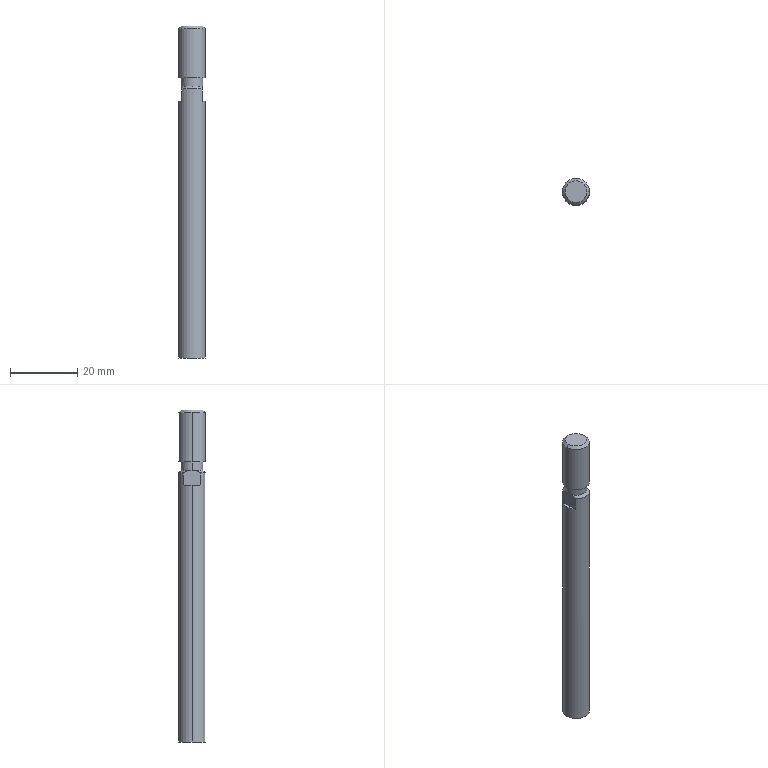Part | NX | features BREP 1 | 1 solid | 19 faces | box 8 x 8 x 99 mm | volume 4889 mm3 | plane 9 | cylinder 6 | cone 4 | commonest cylinder face diameters 8 x4 6.47 x2
STEP:
#1=CARTESIAN_POINT('',(3.,2.646,0.5));
#2=VERTEX_POINT('',#1);
#3=CARTESIAN_POINT('',(4.,0.,0.5));
#4=VERTEX_POINT('',#3);
#5=CARTESIAN_POINT('',(0.,0.,0.5));
#6=DIRECTION('',(0.,0.,-1.));
#7=DIRECTION('',(-1.,0.,0.));
#8=AXIS2_PLACEMENT_3D('',#5,#6,#7);
#9=CIRCLE('',#8,4.);
#10=EDGE_CURVE('',#2,#4,#9,.T.);
#11=ORIENTED_EDGE('',*,*,#10,.T.);
#12=CARTESIAN_POINT('',(4.,0.,-76.));
#13=VERTEX_POINT('',#12);
#14=CARTESIAN_POINT('',(4.,0.,-35.883));
#15=DIRECTION('',(0.,0.,-1.));
#16=VECTOR('',#15,1000.);
#17=LINE('',#14,#16);
#18=EDGE_CURVE('',#4,#13,#17,.T.);
#19=ORIENTED_EDGE('',*,*,#18,.T.);
#20=CARTESIAN_POINT('',(-4.,0.,-76.));
#21=VERTEX_POINT('',#20);
#22=CARTESIAN_POINT('',(0.,0.,-76.));
#23=DIRECTION('',(0.,0.,1.));
#24=DIRECTION('',(-1.,0.,0.));
#25=AXIS2_PLACEMENT_3D('',#22,#23,#24);
#26=CIRCLE('',#25,4.);
#27=EDGE_CURVE('',#13,#21,#26,.T.);
#28=ORIENTED_EDGE('',*,*,#27,.T.);
#29=CARTESIAN_POINT('',(-4.,0.,0.5));
#30=VERTEX_POINT('',#29);
#31=CARTESIAN_POINT('',(-4.,0.,-35.883));
#32=DIRECTION('',(0.,0.,-1.));
#33=VECTOR('',#32,1000.);
#34=LINE('',#31,#33);
#35=EDGE_CURVE('',#30,#21,#34,.T.);
#36=ORIENTED_EDGE('',*,*,#35,.F.);
#37=CARTESIAN_POINT('',(-3.,2.646,0.5));
#38=VERTEX_POINT('',#37);
#39=CARTESIAN_POINT('',(0.,0.,0.5));
#40=DIRECTION('',(0.,0.,-1.));
#41=DIRECTION('',(-1.,0.,0.));
#42=AXIS2_PLACEMENT_3D('',#39,#40,#41);
#43=CIRCLE('',#42,4.);
#44=EDGE_CURVE('',#30,#38,#43,.T.);
#45=ORIENTED_EDGE('',*,*,#44,.T.);
#46=CARTESIAN_POINT('',(-3.,2.646,4.235));
#47=VERTEX_POINT('',#46);
#48=CARTESIAN_POINT('',(-3.,2.646,-35.883));
#49=DIRECTION('',(0.,0.,1.));
#50=VECTOR('',#49,1000.);
#51=LINE('',#48,#50);
#52=EDGE_CURVE('',#38,#47,#51,.T.);
#53=ORIENTED_EDGE('',*,*,#52,.T.);
#54=CARTESIAN_POINT('',(3.,2.646,4.235));
#55=VERTEX_POINT('',#54);
#56=CARTESIAN_POINT('',(0.,0.,4.235));
#57=DIRECTION('',(0.,0.,-1.));
#58=DIRECTION('',(-1.,0.,0.));
#59=AXIS2_PLACEMENT_3D('',#56,#57,#58);
#60=CIRCLE('',#59,4.);
#61=EDGE_CURVE('',#47,#55,#60,.T.);
#62=ORIENTED_EDGE('',*,*,#61,.T.);
#63=CARTESIAN_POINT('',(3.,2.646,-35.883));
#64=DIRECTION('',(0.,0.,-1.));
#65=VECTOR('',#64,1000.);
#66=LINE('',#63,#65);
#67=EDGE_CURVE('',#55,#2,#66,.T.);
#68=ORIENTED_EDGE('',*,*,#67,.T.);
#69=EDGE_LOOP('',(#11,#19,#28,#36,#45,#53,#62,#68));
#70=FACE_BOUND('',#69,.T.);
#71=CARTESIAN_POINT('',(0.,0.,-35.883));
#72=DIRECTION('',(0.,0.,-1.));
#73=DIRECTION('',(-1.,0.,0.));
#74=AXIS2_PLACEMENT_3D('',#71,#72,#73);
#75=CYLINDRICAL_SURFACE('',#74,4.);
#76=ADVANCED_FACE('',(#70),#75,.T.);
#77=CARTESIAN_POINT('',(-3.235,0.,7.5));
#78=VERTEX_POINT('',#77);
#79=CARTESIAN_POINT('',(3.235,0.,7.5));
#80=VERTEX_POINT('',#79);
#81=CARTESIAN_POINT('',(0.,0.,7.5));
#82=DIRECTION('',(0.,0.,-1.));
#83=DIRECTION('',(-1.,0.,0.));
#84=AXIS2_PLACEMENT_3D('',#81,#82,#83);
#85=CIRCLE('',#84,3.235);
#86=EDGE_CURVE('',#78,#80,#85,.T.);
#87=ORIENTED_EDGE('',*,*,#86,.T.);
#88=CARTESIAN_POINT('',(3.235,0.,5.));
#89=VERTEX_POINT('',#88);
#90=CARTESIAN_POINT('',(3.235,0.,6.25));
#91=DIRECTION('',(0.,0.,-1.));
#92=VECTOR('',#91,1000.);
#93=LINE('',#90,#92);
#94=EDGE_CURVE('',#80,#89,#93,.T.);
#95=ORIENTED_EDGE('',*,*,#94,.T.);
#96=CARTESIAN_POINT('',(3.,1.21,5.));
#97=VERTEX_POINT('',#96);
#98=CARTESIAN_POINT('',(0.,0.,5.));
#99=DIRECTION('',(0.,0.,1.));
#100=DIRECTION('',(-1.,0.,0.));
#101=AXIS2_PLACEMENT_3D('',#98,#99,#100);
#102=CIRCLE('',#101,3.235);
#103=EDGE_CURVE('',#89,#97,#102,.T.);
#104=ORIENTED_EDGE('',*,*,#103,.T.);
#105=CARTESIAN_POINT('',(-3.,1.21,5.));
#106=VERTEX_POINT('',#105);
#107=CARTESIAN_POINT('',(0.,0.,5.));
#108=DIRECTION('',(0.,0.,-1.));
#109=DIRECTION('',(0.,1.,0.));
#110=AXIS2_PLACEMENT_3D('',#107,#108,#109);
#111=CIRCLE('',#110,3.235);
#112=EDGE_CURVE('',#106,#97,#111,.T.);
#113=ORIENTED_EDGE('',*,*,#112,.F.);
#114=CARTESIAN_POINT('',(-3.235,0.,5.));
#115=VERTEX_POINT('',#114);
#116=CARTESIAN_POINT('',(0.,0.,5.));
#117=DIRECTION('',(0.,0.,1.));
#118=DIRECTION('',(-1.,0.,0.));
#119=AXIS2_PLACEMENT_3D('',#116,#117,#118);
#120=CIRCLE('',#119,3.235);
#121=EDGE_CURVE('',#106,#115,#120,.T.);
#122=ORIENTED_EDGE('',*,*,#121,.T.);
#123=CARTESIAN_POINT('',(-3.235,0.,6.25));
#124=DIRECTION('',(0.,0.,-1.));
#125=VECTOR('',#124,1000.);
#126=LINE('',#123,#125);
#127=EDGE_CURVE('',#78,#115,#126,.T.);
#128=ORIENTED_EDGE('',*,*,#127,.F.);
#129=EDGE_LOOP('',(#87,#95,#104,#113,#122,#128));
#130=FACE_BOUND('',#129,.T.);
#131=CARTESIAN_POINT('',(0.,0.,6.25));
#132=DIRECTION('',(0.,0.,-1.));
#133=DIRECTION('',(-1.,0.,0.));
#134=AXIS2_PLACEMENT_3D('',#131,#132,#133);
#135=CYLINDRICAL_SURFACE('',#134,3.235);
#136=ADVANCED_FACE('',(#130),#135,.T.);
#137=CARTESIAN_POINT('',(-4.,0.,22.235));
#138=VERTEX_POINT('',#137);
#139=CARTESIAN_POINT('',(4.,0.,22.235));
#140=VERTEX_POINT('',#139);
#141=CARTESIAN_POINT('',(0.,0.,22.235));
#142=DIRECTION('',(0.,0.,-1.));
#143=DIRECTION('',(-1.,0.,0.));
#144=AXIS2_PLACEMENT_3D('',#141,#142,#143);
#145=CIRCLE('',#144,4.);
#146=EDGE_CURVE('',#138,#140,#145,.T.);
#147=ORIENTED_EDGE('',*,*,#146,.T.);
#148=CARTESIAN_POINT('',(4.,0.,7.5));
#149=VERTEX_POINT('',#148);
#150=CARTESIAN_POINT('',(4.,0.,14.867));
#151=DIRECTION('',(0.,0.,-1.));
#152=VECTOR('',#151,1000.);
#153=LINE('',#150,#152);
#154=EDGE_CURVE('',#140,#149,#153,.T.);
#155=ORIENTED_EDGE('',*,*,#154,.T.);
#156=CARTESIAN_POINT('',(-4.,0.,7.5));
#157=VERTEX_POINT('',#156);
#158=CARTESIAN_POINT('',(0.,0.,7.5));
#159=DIRECTION('',(0.,0.,-1.));
#160=DIRECTION('',(-1.,0.,0.));
#161=AXIS2_PLACEMENT_3D('',#158,#159,#160);
#162=CIRCLE('',#161,4.);
#163=EDGE_CURVE('',#157,#149,#162,.T.);
#164=ORIENTED_EDGE('',*,*,#163,.F.);
#165=CARTESIAN_POINT('',(-4.,0.,14.867));
#166=DIRECTION('',(0.,0.,-1.));
#167=VECTOR('',#166,1000.);
#168=LINE('',#165,#167);
#169=EDGE_CURVE('',#138,#157,#168,.T.);
#170=ORIENTED_EDGE('',*,*,#169,.F.);
#171=EDGE_LOOP('',(#147,#155,#164,#170));
#172=FACE_BOUND('',#171,.T.);
#173=CARTESIAN_POINT('',(0.,0.,14.867));
#174=DIRECTION('',(0.,0.,-1.));
#175=DIRECTION('',(-1.,0.,0.));
#176=AXIS2_PLACEMENT_3D('',#173,#174,#175);
#177=CYLINDRICAL_SURFACE('',#176,4.);
#178=ADVANCED_FACE('',(#172),#177,.T.);
#179=CARTESIAN_POINT('',(-3.235,0.,23.));
#180=VERTEX_POINT('',#179);
#181=CARTESIAN_POINT('',(3.235,0.,23.));
#182=VERTEX_POINT('',#181);
#183=CARTESIAN_POINT('',(0.,0.,23.));
#184=DIRECTION('',(0.,0.,-1.));
#185=DIRECTION('',(-1.,0.,0.));
#186=AXIS2_PLACEMENT_3D('',#183,#184,#185);
#187=CIRCLE('',#186,3.235);
#188=EDGE_CURVE('',#180,#182,#187,.T.);
#189=ORIENTED_EDGE('',*,*,#188,.T.);
#190=CARTESIAN_POINT('',(4.,0.,22.235));
#191=DIRECTION('',(0.7071,0.,-0.7071));
#192=VECTOR('',#191,1000.);
#193=LINE('',#190,#192);
#194=EDGE_CURVE('',#182,#140,#193,.T.);
#195=ORIENTED_EDGE('',*,*,#194,.T.);
#196=ORIENTED_EDGE('',*,*,#146,.F.);
#197=CARTESIAN_POINT('',(-4.,0.,22.235));
#198=DIRECTION('',(-0.7071,0.,-0.7071));
#199=VECTOR('',#198,1000.);
#200=LINE('',#197,#199);
#201=EDGE_CURVE('',#180,#138,#200,.T.);
#202=ORIENTED_EDGE('',*,*,#201,.F.);
#203=EDGE_LOOP('',(#189,#195,#196,#202));
#204=FACE_BOUND('',#203,.T.);
#205=CARTESIAN_POINT('',(0.,0.,22.235));
#206=DIRECTION('',(0.,0.,-1.));
#207=DIRECTION('',(-1.,0.,0.));
#208=AXIS2_PLACEMENT_3D('',#205,#206,#207);
#209=CONICAL_SURFACE('',#208,4.,0.7854);
#210=ADVANCED_FACE('',(#204),#209,.T.);
#211=ORIENTED_EDGE('',*,*,#18,.F.);
#212=CARTESIAN_POINT('',(3.,-2.646,0.5));
#213=VERTEX_POINT('',#212);
#214=CARTESIAN_POINT('',(0.,0.,0.5));
#215=DIRECTION('',(0.,0.,-1.));
#216=DIRECTION('',(-1.,0.,0.));
#217=AXIS2_PLACEMENT_3D('',#214,#215,#216);
#218=CIRCLE('',#217,4.);
#219=EDGE_CURVE('',#4,#213,#218,.T.);
#220=ORIENTED_EDGE('',*,*,#219,.T.);
#221=CARTESIAN_POINT('',(3.,-2.646,4.235));
#222=VERTEX_POINT('',#221);
#223=CARTESIAN_POINT('',(3.,-2.646,-35.883));
#224=DIRECTION('',(0.,0.,1.));
#225=VECTOR('',#224,1000.);
#226=LINE('',#223,#225);
#227=EDGE_CURVE('',#213,#222,#226,.T.);
#228=ORIENTED_EDGE('',*,*,#227,.T.);
#229=CARTESIAN_POINT('',(-3.,-2.646,4.235));
#230=VERTEX_POINT('',#229);
#231=CARTESIAN_POINT('',(0.,0.,4.235));
#232=DIRECTION('',(0.,0.,-1.));
#233=DIRECTION('',(-1.,0.,0.));
#234=AXIS2_PLACEMENT_3D('',#231,#232,#233);
#235=CIRCLE('',#234,4.);
#236=EDGE_CURVE('',#222,#230,#235,.T.);
#237=ORIENTED_EDGE('',*,*,#236,.T.);
#238=CARTESIAN_POINT('',(-3.,-2.646,0.5));
#239=VERTEX_POINT('',#238);
#240=CARTESIAN_POINT('',(-3.,-2.646,-35.883));
#241=DIRECTION('',(0.,0.,-1.));
#242=VECTOR('',#241,1000.);
#243=LINE('',#240,#242);
#244=EDGE_CURVE('',#230,#239,#243,.T.);
#245=ORIENTED_EDGE('',*,*,#244,.T.);
#246=CARTESIAN_POINT('',(0.,0.,0.5));
#247=DIRECTION('',(0.,0.,-1.));
#248=DIRECTION('',(-1.,0.,0.));
#249=AXIS2_PLACEMENT_3D('',#246,#247,#248);
#250=CIRCLE('',#249,4.);
#251=EDGE_CURVE('',#239,#30,#250,.T.);
#252=ORIENTED_EDGE('',*,*,#251,.T.);
#253=ORIENTED_EDGE('',*,*,#35,.T.);
#254=CARTESIAN_POINT('',(0.,0.,-76.));
#255=DIRECTION('',(0.,0.,1.));
#256=DIRECTION('',(-1.,0.,0.));
#257=AXIS2_PLACEMENT_3D('',#254,#255,#256);
#258=CIRCLE('',#257,4.);
#259=EDGE_CURVE('',#21,#13,#258,.T.);
#260=ORIENTED_EDGE('',*,*,#259,.T.);
#261=EDGE_LOOP('',(#211,#220,#228,#237,#245,#252,#253,#260));
#262=FACE_BOUND('',#261,.T.);
#263=CARTESIAN_POINT('',(0.,0.,-35.883));
#264=DIRECTION('',(0.,0.,-1.));
#265=DIRECTION('',(-1.,0.,0.));
#266=AXIS2_PLACEMENT_3D('',#263,#264,#265);
#267=CYLINDRICAL_SURFACE('',#266,4.);
#268=ADVANCED_FACE('',(#262),#267,.T.);
#269=CARTESIAN_POINT('',(-3.,1.21,5.));
#270=CARTESIAN_POINT('',(-3.,1.653,4.834));
#271=CARTESIAN_POINT('',(-3.,2.119,4.584));
#272=CARTESIAN_POINT('',(-3.,2.646,4.235));
#273=B_SPLINE_CURVE_WITH_KNOTS('',3,(#269,#270,#271,#272),.UNSPECIFIED.,.F.,.F.,(4,4),(0.,1.),.UNSPECIFIED.);
#274=EDGE_CURVE('',#47,#106,#273,.F.);
#275=ORIENTED_EDGE('',*,*,#274,.T.);
#276=ORIENTED_EDGE('',*,*,#112,.T.);
#277=CARTESIAN_POINT('',(3.,2.646,4.235));
#278=CARTESIAN_POINT('',(3.,2.12,4.583));
#279=CARTESIAN_POINT('',(3.,1.654,4.834));
#280=CARTESIAN_POINT('',(3.,1.21,5.));
#281=B_SPLINE_CURVE_WITH_KNOTS('',3,(#277,#278,#279,#280),.UNSPECIFIED.,.F.,.F.,(4,4),(0.,1.),.UNSPECIFIED.);
#282=EDGE_CURVE('',#97,#55,#281,.F.);
#283=ORIENTED_EDGE('',*,*,#282,.T.);
#284=ORIENTED_EDGE('',*,*,#61,.F.);
#285=EDGE_LOOP('',(#275,#276,#283,#284));
#286=FACE_BOUND('',#285,.T.);
#287=CARTESIAN_POINT('',(0.,0.,4.235));
#288=DIRECTION('',(0.,0.,-1.));
#289=DIRECTION('',(-1.,0.,0.));
#290=AXIS2_PLACEMENT_3D('',#287,#288,#289);
#291=CONICAL_SURFACE('',#290,4.,0.7854);
#292=ADVANCED_FACE('',(#286),#291,.T.);
#293=CARTESIAN_POINT('',(-3.,-1.21,5.));
#294=VERTEX_POINT('',#293);
#295=CARTESIAN_POINT('',(-3.,8.,5.));
#296=DIRECTION('',(0.,-1.,0.));
#297=VECTOR('',#296,1000.);
#298=LINE('',#295,#297);
#299=EDGE_CURVE('',#106,#294,#298,.T.);
#300=ORIENTED_EDGE('',*,*,#299,.F.);
#301=ORIENTED_EDGE('',*,*,#274,.F.);
#302=ORIENTED_EDGE('',*,*,#52,.F.);
#303=CARTESIAN_POINT('',(-3.,8.,0.5));
#304=DIRECTION('',(0.,1.,0.));
#305=VECTOR('',#304,1000.);
#306=LINE('',#303,#305);
#307=EDGE_CURVE('',#239,#38,#306,.T.);
#308=ORIENTED_EDGE('',*,*,#307,.F.);
#309=ORIENTED_EDGE('',*,*,#244,.F.);
#310=CARTESIAN_POINT('',(-3.,-2.646,4.235));
#311=CARTESIAN_POINT('',(-3.,-2.12,4.583));
#312=CARTESIAN_POINT('',(-3.,-1.654,4.834));
#313=CARTESIAN_POINT('',(-3.,-1.21,5.));
#314=B_SPLINE_CURVE_WITH_KNOTS('',3,(#310,#311,#312,#313),.UNSPECIFIED.,.F.,.F.,(4,4),(0.,1.),.UNSPECIFIED.);
#315=EDGE_CURVE('',#294,#230,#314,.F.);
#316=ORIENTED_EDGE('',*,*,#315,.F.);
#317=EDGE_LOOP('',(#300,#301,#302,#308,#309,#316));
#318=FACE_BOUND('',#317,.T.);
#319=CARTESIAN_POINT('',(-3.,8.,5.));
#320=DIRECTION('',(1.,0.,0.));
#321=DIRECTION('',(0.,1.,0.));
#322=AXIS2_PLACEMENT_3D('',#319,#320,#321);
#323=PLANE('',#322);
#324=ADVANCED_FACE('',(#318),#323,.F.);
#325=ORIENTED_EDGE('',*,*,#307,.T.);
#326=ORIENTED_EDGE('',*,*,#44,.F.);
#327=ORIENTED_EDGE('',*,*,#251,.F.);
#328=EDGE_LOOP('',(#325,#326,#327));
#329=FACE_BOUND('',#328,.T.);
#330=CARTESIAN_POINT('',(-3.,8.,0.5));
#331=DIRECTION('',(0.,0.,-1.));
#332=DIRECTION('',(0.,-1.,0.));
#333=AXIS2_PLACEMENT_3D('',#330,#331,#332);
#334=PLANE('',#333);
#335=ADVANCED_FACE('',(#329),#334,.F.);
#336=ORIENTED_EDGE('',*,*,#315,.T.);
#337=ORIENTED_EDGE('',*,*,#236,.F.);
#338=CARTESIAN_POINT('',(3.,-1.21,5.));
#339=VERTEX_POINT('',#338);
#340=CARTESIAN_POINT('',(3.,-1.21,5.));
#341=CARTESIAN_POINT('',(3.,-1.653,4.834));
#342=CARTESIAN_POINT('',(3.,-2.119,4.584));
#343=CARTESIAN_POINT('',(3.,-2.646,4.235));
#344=B_SPLINE_CURVE_WITH_KNOTS('',3,(#340,#341,#342,#343),.UNSPECIFIED.,.F.,.F.,(4,4),(0.,1.),.UNSPECIFIED.);
#345=EDGE_CURVE('',#222,#339,#344,.F.);
#346=ORIENTED_EDGE('',*,*,#345,.T.);
#347=CARTESIAN_POINT('',(0.,0.,5.));
#348=DIRECTION('',(0.,0.,-1.));
#349=DIRECTION('',(0.,1.,0.));
#350=AXIS2_PLACEMENT_3D('',#347,#348,#349);
#351=CIRCLE('',#350,3.235);
#352=EDGE_CURVE('',#339,#294,#351,.T.);
#353=ORIENTED_EDGE('',*,*,#352,.T.);
#354=EDGE_LOOP('',(#336,#337,#346,#353));
#355=FACE_BOUND('',#354,.T.);
#356=CARTESIAN_POINT('',(0.,0.,4.235));
#357=DIRECTION('',(0.,0.,-1.));
#358=DIRECTION('',(-1.,0.,0.));
#359=AXIS2_PLACEMENT_3D('',#356,#357,#358);
#360=CONICAL_SURFACE('',#359,4.,0.7854);
#361=ADVANCED_FACE('',(#355),#360,.T.);
#362=ORIENTED_EDGE('',*,*,#259,.F.);
#363=ORIENTED_EDGE('',*,*,#27,.F.);
#364=EDGE_LOOP('',(#362,#363));
#365=FACE_BOUND('',#364,.T.);
#366=CARTESIAN_POINT('',(0.,2.,-76.));
#367=DIRECTION('',(0.,0.,-1.));
#368=DIRECTION('',(0.,-1.,0.));
#369=AXIS2_PLACEMENT_3D('',#366,#367,#368);
#370=PLANE('',#369);
#371=ADVANCED_FACE('',(#365),#370,.T.);
#372=ORIENTED_EDGE('',*,*,#94,.F.);
#373=CARTESIAN_POINT('',(0.,0.,7.5));
#374=DIRECTION('',(0.,0.,-1.));
#375=DIRECTION('',(-1.,0.,0.));
#376=AXIS2_PLACEMENT_3D('',#373,#374,#375);
#377=CIRCLE('',#376,3.235);
#378=EDGE_CURVE('',#80,#78,#377,.T.);
#379=ORIENTED_EDGE('',*,*,#378,.T.);
#380=ORIENTED_EDGE('',*,*,#127,.T.);
#381=CARTESIAN_POINT('',(0.,0.,5.));
#382=DIRECTION('',(0.,0.,1.));
#383=DIRECTION('',(-1.,0.,0.));
#384=AXIS2_PLACEMENT_3D('',#381,#382,#383);
#385=CIRCLE('',#384,3.235);
#386=EDGE_CURVE('',#115,#294,#385,.T.);
#387=ORIENTED_EDGE('',*,*,#386,.T.);
#388=ORIENTED_EDGE('',*,*,#352,.F.);
#389=CARTESIAN_POINT('',(0.,0.,5.));
#390=DIRECTION('',(0.,0.,1.));
#391=DIRECTION('',(-1.,0.,0.));
#392=AXIS2_PLACEMENT_3D('',#389,#390,#391);
#393=CIRCLE('',#392,3.235);
#394=EDGE_CURVE('',#339,#89,#393,.T.);
#395=ORIENTED_EDGE('',*,*,#394,.T.);
#396=EDGE_LOOP('',(#372,#379,#380,#387,#388,#395));
#397=FACE_BOUND('',#396,.T.);
#398=CARTESIAN_POINT('',(0.,0.,6.25));
#399=DIRECTION('',(0.,0.,-1.));
#400=DIRECTION('',(-1.,0.,0.));
#401=AXIS2_PLACEMENT_3D('',#398,#399,#400);
#402=CYLINDRICAL_SURFACE('',#401,3.235);
#403=ADVANCED_FACE('',(#397),#402,.T.);
#404=ORIENTED_EDGE('',*,*,#299,.T.);
#405=ORIENTED_EDGE('',*,*,#386,.F.);
#406=ORIENTED_EDGE('',*,*,#121,.F.);
#407=EDGE_LOOP('',(#404,#405,#406));
#408=FACE_BOUND('',#407,.T.);
#409=CARTESIAN_POINT('',(-6.,8.,5.));
#410=DIRECTION('',(0.,0.,1.));
#411=DIRECTION('',(1.,0.,0.));
#412=AXIS2_PLACEMENT_3D('',#409,#410,#411);
#413=PLANE('',#412);
#414=ADVANCED_FACE('',(#408),#413,.F.);
#415=ORIENTED_EDGE('',*,*,#227,.F.);
#416=CARTESIAN_POINT('',(3.,8.,0.5));
#417=DIRECTION('',(0.,-1.,0.));
#418=VECTOR('',#417,1000.);
#419=LINE('',#416,#418);
#420=EDGE_CURVE('',#2,#213,#419,.T.);
#421=ORIENTED_EDGE('',*,*,#420,.F.);
#422=ORIENTED_EDGE('',*,*,#67,.F.);
#423=ORIENTED_EDGE('',*,*,#282,.F.);
#424=CARTESIAN_POINT('',(3.,8.,5.));
#425=DIRECTION('',(0.,1.,0.));
#426=VECTOR('',#425,1000.);
#427=LINE('',#424,#426);
#428=EDGE_CURVE('',#339,#97,#427,.T.);
#429=ORIENTED_EDGE('',*,*,#428,.F.);
#430=ORIENTED_EDGE('',*,*,#345,.F.);
#431=EDGE_LOOP('',(#415,#421,#422,#423,#429,#430));
#432=FACE_BOUND('',#431,.T.);
#433=CARTESIAN_POINT('',(3.,8.,0.5));
#434=DIRECTION('',(-1.,0.,0.));
#435=DIRECTION('',(0.,0.,1.));
#436=AXIS2_PLACEMENT_3D('',#433,#434,#435);
#437=PLANE('',#436);
#438=ADVANCED_FACE('',(#432),#437,.F.);
#439=ORIENTED_EDGE('',*,*,#420,.T.);
#440=ORIENTED_EDGE('',*,*,#219,.F.);
#441=ORIENTED_EDGE('',*,*,#10,.F.);
#442=EDGE_LOOP('',(#439,#440,#441));
#443=FACE_BOUND('',#442,.T.);
#444=CARTESIAN_POINT('',(6.,8.,0.5));
#445=DIRECTION('',(0.,0.,-1.));
#446=DIRECTION('',(0.,-1.,0.));
#447=AXIS2_PLACEMENT_3D('',#444,#445,#446);
#448=PLANE('',#447);
#449=ADVANCED_FACE('',(#443),#448,.F.);
#450=ORIENTED_EDGE('',*,*,#163,.T.);
#451=CARTESIAN_POINT('',(0.,0.,7.5));
#452=DIRECTION('',(0.,0.,-1.));
#453=DIRECTION('',(-1.,0.,0.));
#454=AXIS2_PLACEMENT_3D('',#451,#452,#453);
#455=CIRCLE('',#454,4.);
#456=EDGE_CURVE('',#149,#157,#455,.T.);
#457=ORIENTED_EDGE('',*,*,#456,.T.);
#458=EDGE_LOOP('',(#450,#457));
#459=FACE_BOUND('',#458,.T.);
#460=ORIENTED_EDGE('',*,*,#86,.F.);
#461=ORIENTED_EDGE('',*,*,#378,.F.);
#462=EDGE_LOOP('',(#460,#461));
#463=FACE_BOUND('',#462,.T.);
#464=CARTESIAN_POINT('',(0.,3.618,7.5));
#465=DIRECTION('',(0.,0.,-1.));
#466=DIRECTION('',(0.,-1.,0.));
#467=AXIS2_PLACEMENT_3D('',#464,#465,#466);
#468=PLANE('',#467);
#469=ADVANCED_FACE('',(#459,#463),#468,.T.);
#470=ORIENTED_EDGE('',*,*,#428,.T.);
#471=ORIENTED_EDGE('',*,*,#103,.F.);
#472=ORIENTED_EDGE('',*,*,#394,.F.);
#473=EDGE_LOOP('',(#470,#471,#472));
#474=FACE_BOUND('',#473,.T.);
#475=CARTESIAN_POINT('',(3.,8.,5.));
#476=DIRECTION('',(0.,0.,1.));
#477=DIRECTION('',(1.,0.,0.));
#478=AXIS2_PLACEMENT_3D('',#475,#476,#477);
#479=PLANE('',#478);
#480=ADVANCED_FACE('',(#474),#479,.F.);
#481=ORIENTED_EDGE('',*,*,#154,.F.);
#482=CARTESIAN_POINT('',(0.,0.,22.235));
#483=DIRECTION('',(0.,0.,-1.));
#484=DIRECTION('',(-1.,0.,0.));
#485=AXIS2_PLACEMENT_3D('',#482,#483,#484);
#486=CIRCLE('',#485,4.);
#487=EDGE_CURVE('',#140,#138,#486,.T.);
#488=ORIENTED_EDGE('',*,*,#487,.T.);
#489=ORIENTED_EDGE('',*,*,#169,.T.);
#490=ORIENTED_EDGE('',*,*,#456,.F.);
#491=EDGE_LOOP('',(#481,#488,#489,#490));
#492=FACE_BOUND('',#491,.T.);
#493=CARTESIAN_POINT('',(0.,0.,14.867));
#494=DIRECTION('',(0.,0.,-1.));
#495=DIRECTION('',(-1.,0.,0.));
#496=AXIS2_PLACEMENT_3D('',#493,#494,#495);
#497=CYLINDRICAL_SURFACE('',#496,4.);
#498=ADVANCED_FACE('',(#492),#497,.T.);
#499=ORIENTED_EDGE('',*,*,#194,.F.);
#500=CARTESIAN_POINT('',(0.,0.,23.));
#501=DIRECTION('',(0.,0.,-1.));
#502=DIRECTION('',(-1.,0.,0.));
#503=AXIS2_PLACEMENT_3D('',#500,#501,#502);
#504=CIRCLE('',#503,3.235);
#505=EDGE_CURVE('',#182,#180,#504,.T.);
#506=ORIENTED_EDGE('',*,*,#505,.T.);
#507=ORIENTED_EDGE('',*,*,#201,.T.);
#508=ORIENTED_EDGE('',*,*,#487,.F.);
#509=EDGE_LOOP('',(#499,#506,#507,#508));
#510=FACE_BOUND('',#509,.T.);
#511=CARTESIAN_POINT('',(0.,0.,22.235));
#512=DIRECTION('',(0.,0.,-1.));
#513=DIRECTION('',(-1.,0.,0.));
#514=AXIS2_PLACEMENT_3D('',#511,#512,#513);
#515=CONICAL_SURFACE('',#514,4.,0.7854);
#516=ADVANCED_FACE('',(#510),#515,.T.);
#517=ORIENTED_EDGE('',*,*,#188,.F.);
#518=ORIENTED_EDGE('',*,*,#505,.F.);
#519=EDGE_LOOP('',(#517,#518));
#520=FACE_BOUND('',#519,.T.);
#521=CARTESIAN_POINT('',(0.,1.617,23.));
#522=DIRECTION('',(0.,0.,1.));
#523=DIRECTION('',(1.,0.,0.));
#524=AXIS2_PLACEMENT_3D('',#521,#522,#523);
#525=PLANE('',#524);
#526=ADVANCED_FACE('',(#520),#525,.T.);
#527=CLOSED_SHELL('',(#76,#136,#178,#210,#268,#292,#324,#335,#361,#371,#403,#414,#438,#449,#469,#480,#498,#516,#526));
#528=MANIFOLD_SOLID_BREP('',#527);
#529=(LENGTH_UNIT()NAMED_UNIT(*)SI_UNIT(.MILLI.,.METRE.));
#530=UNCERTAINTY_MEASURE_WITH_UNIT(LENGTH_MEASURE(0.0508),#529,'','');
#531=(NAMED_UNIT(*)PLANE_ANGLE_UNIT()SI_UNIT($,.RADIAN.));
#532=(NAMED_UNIT(*)SI_UNIT($,.STERADIAN.)SOLID_ANGLE_UNIT());
#533=(GEOMETRIC_REPRESENTATION_CONTEXT(3)GLOBAL_UNCERTAINTY_ASSIGNED_CONTEXT((#530))GLOBAL_UNIT_ASSIGNED_CONTEXT((#529,#531,#532))REPRESENTATION_CONTEXT('',''));
#534=ADVANCED_BREP_SHAPE_REPRESENTATION('',(#528),#533);